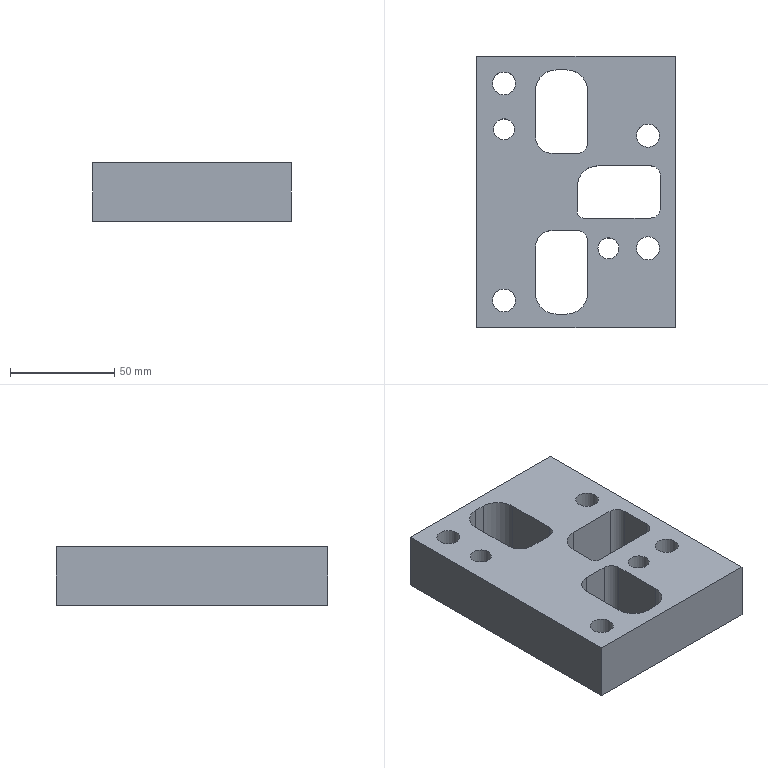Part | STEP file | PN_0015_id866_x_t | 1 solid | 44 faces | box 95 x 130 x 28 mm | volume 241686 mm3 | plane 22 | cylinder 22 | commonest cylinder face diameters 10 x6 20 x5 11 x4 17 x4 16 x2 6 x1
STEP:
#1=CARTESIAN_POINT('',(-190.55,-65.,95.));
#2=VERTEX_POINT('',#1);
#3=CARTESIAN_POINT('',(-190.55,65.,95.));
#4=VERTEX_POINT('',#3);
#5=CARTESIAN_POINT('',(-190.55,0.,95.));
#6=DIRECTION('',(0.,1.,0.));
#7=VECTOR('',#6,1.);
#8=LINE('',#5,#7);
#9=EDGE_CURVE('',#2,#4,#8,.T.);
#10=ORIENTED_EDGE('',*,*,#9,.F.);
#11=CARTESIAN_POINT('',(-190.55,-65.,67.));
#12=VERTEX_POINT('',#11);
#13=CARTESIAN_POINT('',(-190.55,-65.,-36.));
#14=DIRECTION('',(0.,0.,1.));
#15=VECTOR('',#14,1.);
#16=LINE('',#13,#15);
#17=EDGE_CURVE('',#12,#2,#16,.T.);
#18=ORIENTED_EDGE('',*,*,#17,.F.);
#19=CARTESIAN_POINT('',(-190.55,65.,67.));
#20=VERTEX_POINT('',#19);
#21=CARTESIAN_POINT('',(-190.55,0.,67.));
#22=DIRECTION('',(0.,1.,0.));
#23=VECTOR('',#22,1.);
#24=LINE('',#21,#23);
#25=EDGE_CURVE('',#12,#20,#24,.T.);
#26=ORIENTED_EDGE('',*,*,#25,.T.);
#27=CARTESIAN_POINT('',(-190.55,65.,-36.));
#28=DIRECTION('',(0.,0.,1.));
#29=VECTOR('',#28,1.);
#30=LINE('',#27,#29);
#31=EDGE_CURVE('',#20,#4,#30,.T.);
#32=ORIENTED_EDGE('',*,*,#31,.T.);
#33=EDGE_LOOP('',(#10,#18,#26,#32));
#34=FACE_OUTER_BOUND('',#33,.T.);
#35=CARTESIAN_POINT('',(-190.55,0.,-36.));
#36=DIRECTION('',(-1.,0.,0.));
#37=DIRECTION('',(0.,1.,0.));
#38=AXIS2_PLACEMENT_3D('',#35,#36,#37);
#39=PLANE('',#38);
#40=ADVANCED_FACE('',(#34),#39,.F.);
#41=CARTESIAN_POINT('',(-285.55,-65.,67.));
#42=VERTEX_POINT('',#41);
#43=CARTESIAN_POINT('',(-224.,-65.,67.));
#44=DIRECTION('',(1.,0.,0.));
#45=VECTOR('',#44,1.);
#46=LINE('',#43,#45);
#47=EDGE_CURVE('',#42,#12,#46,.T.);
#48=ORIENTED_EDGE('',*,*,#47,.T.);
#49=ORIENTED_EDGE('',*,*,#17,.T.);
#50=CARTESIAN_POINT('',(-285.55,-65.,95.));
#51=VERTEX_POINT('',#50);
#52=CARTESIAN_POINT('',(-224.,-65.,95.));
#53=DIRECTION('',(1.,0.,0.));
#54=VECTOR('',#53,1.);
#55=LINE('',#52,#54);
#56=EDGE_CURVE('',#51,#2,#55,.T.);
#57=ORIENTED_EDGE('',*,*,#56,.F.);
#58=CARTESIAN_POINT('',(-285.55,-65.,-36.));
#59=DIRECTION('',(0.,0.,1.));
#60=VECTOR('',#59,1.);
#61=LINE('',#58,#60);
#62=EDGE_CURVE('',#42,#51,#61,.T.);
#63=ORIENTED_EDGE('',*,*,#62,.F.);
#64=EDGE_LOOP('',(#48,#49,#57,#63));
#65=FACE_OUTER_BOUND('',#64,.T.);
#66=CARTESIAN_POINT('',(-224.,-65.,-36.));
#67=DIRECTION('',(0.,-1.,0.));
#68=DIRECTION('',(-1.,0.,0.));
#69=AXIS2_PLACEMENT_3D('',#66,#67,#68);
#70=PLANE('',#69);
#71=ADVANCED_FACE('',(#65),#70,.T.);
#72=ORIENTED_EDGE('',*,*,#56,.T.);
#73=ORIENTED_EDGE('',*,*,#9,.T.);
#74=CARTESIAN_POINT('',(-285.55,65.,95.));
#75=VERTEX_POINT('',#74);
#76=CARTESIAN_POINT('',(-119.811,65.,95.));
#77=DIRECTION('',(1.,0.,0.));
#78=VECTOR('',#77,1.);
#79=LINE('',#76,#78);
#80=EDGE_CURVE('',#75,#4,#79,.T.);
#81=ORIENTED_EDGE('',*,*,#80,.F.);
#82=CARTESIAN_POINT('',(-285.55,0.,95.));
#83=DIRECTION('',(0.,-1.,0.));
#84=VECTOR('',#83,1.);
#85=LINE('',#82,#84);
#86=EDGE_CURVE('',#75,#51,#85,.T.);
#87=ORIENTED_EDGE('',*,*,#86,.T.);
#88=EDGE_LOOP('',(#72,#73,#81,#87));
#89=FACE_BOUND('',#88,.T.);
#90=CARTESIAN_POINT('',(-267.05,52.,95.));
#91=VERTEX_POINT('',#90);
#92=CARTESIAN_POINT('',(-272.55,52.,95.));
#93=DIRECTION('',(0.,0.,-1.));
#94=DIRECTION('',(1.,0.,0.));
#95=AXIS2_PLACEMENT_3D('',#92,#93,#94);
#96=CIRCLE('',#95,5.5);
#97=EDGE_CURVE('',#91,#91,#96,.T.);
#98=ORIENTED_EDGE('',*,*,#97,.T.);
#99=EDGE_LOOP('',(#98));
#100=FACE_BOUND('',#99,.T.);
#101=CARTESIAN_POINT('',(-267.05,-52.,95.));
#102=VERTEX_POINT('',#101);
#103=CARTESIAN_POINT('',(-272.55,-52.,95.));
#104=DIRECTION('',(0.,0.,-1.));
#105=DIRECTION('',(1.,0.,0.));
#106=AXIS2_PLACEMENT_3D('',#103,#104,#105);
#107=CIRCLE('',#106,5.5);
#108=EDGE_CURVE('',#102,#102,#107,.T.);
#109=ORIENTED_EDGE('',*,*,#108,.T.);
#110=EDGE_LOOP('',(#109));
#111=FACE_BOUND('',#110,.T.);
#112=CARTESIAN_POINT('',(-198.05,-27.,95.));
#113=VERTEX_POINT('',#112);
#114=CARTESIAN_POINT('',(-203.55,-27.,95.));
#115=DIRECTION('',(0.,0.,-1.));
#116=DIRECTION('',(1.,0.,0.));
#117=AXIS2_PLACEMENT_3D('',#114,#115,#116);
#118=CIRCLE('',#117,5.5);
#119=EDGE_CURVE('',#113,#113,#118,.T.);
#120=ORIENTED_EDGE('',*,*,#119,.T.);
#121=EDGE_LOOP('',(#120));
#122=FACE_BOUND('',#121,.T.);
#123=CARTESIAN_POINT('',(-198.05,27.,95.));
#124=VERTEX_POINT('',#123);
#125=CARTESIAN_POINT('',(-203.55,27.,95.));
#126=DIRECTION('',(0.,0.,-1.));
#127=DIRECTION('',(1.,0.,0.));
#128=AXIS2_PLACEMENT_3D('',#125,#126,#127);
#129=CIRCLE('',#128,5.5);
#130=EDGE_CURVE('',#124,#124,#129,.T.);
#131=ORIENTED_EDGE('',*,*,#130,.T.);
#132=EDGE_LOOP('',(#131));
#133=FACE_BOUND('',#132,.T.);
#134=CARTESIAN_POINT('',(-227.5,12.5,95.));
#135=VERTEX_POINT('',#134);
#136=CARTESIAN_POINT('',(-237.5,2.5,95.));
#137=VERTEX_POINT('',#136);
#138=CARTESIAN_POINT('',(-227.5,2.5,95.));
#139=DIRECTION('',(0.,0.,1.));
#140=DIRECTION('',(1.,0.,0.));
#141=AXIS2_PLACEMENT_3D('',#138,#139,#140);
#142=CIRCLE('',#141,10.);
#143=EDGE_CURVE('',#135,#137,#142,.T.);
#144=ORIENTED_EDGE('',*,*,#143,.F.);
#145=CARTESIAN_POINT('',(-202.5,12.5,95.));
#146=VERTEX_POINT('',#145);
#147=CARTESIAN_POINT('',(-209.,12.5,95.));
#148=DIRECTION('',(1.,0.,0.));
#149=VECTOR('',#148,1.);
#150=LINE('',#147,#149);
#151=EDGE_CURVE('',#135,#146,#150,.T.);
#152=ORIENTED_EDGE('',*,*,#151,.T.);
#153=CARTESIAN_POINT('',(-197.5,7.5,95.));
#154=VERTEX_POINT('',#153);
#155=CARTESIAN_POINT('',(-202.5,7.5,95.));
#156=DIRECTION('',(0.,0.,1.));
#157=DIRECTION('',(1.,0.,0.));
#158=AXIS2_PLACEMENT_3D('',#155,#156,#157);
#159=CIRCLE('',#158,5.);
#160=EDGE_CURVE('',#154,#146,#159,.T.);
#161=ORIENTED_EDGE('',*,*,#160,.F.);
#162=CARTESIAN_POINT('',(-197.5,-7.5,95.));
#163=VERTEX_POINT('',#162);
#164=CARTESIAN_POINT('',(-197.5,0.,95.));
#165=DIRECTION('',(0.,-1.,0.));
#166=VECTOR('',#165,1.);
#167=LINE('',#164,#166);
#168=EDGE_CURVE('',#154,#163,#167,.T.);
#169=ORIENTED_EDGE('',*,*,#168,.T.);
#170=CARTESIAN_POINT('',(-202.5,-12.5,95.));
#171=VERTEX_POINT('',#170);
#172=CARTESIAN_POINT('',(-202.5,-7.5,95.));
#173=DIRECTION('',(0.,0.,1.));
#174=DIRECTION('',(1.,0.,0.));
#175=AXIS2_PLACEMENT_3D('',#172,#173,#174);
#176=CIRCLE('',#175,5.);
#177=EDGE_CURVE('',#171,#163,#176,.T.);
#178=ORIENTED_EDGE('',*,*,#177,.F.);
#179=CARTESIAN_POINT('',(-234.5,-12.5,95.));
#180=VERTEX_POINT('',#179);
#181=CARTESIAN_POINT('',(-209.,-12.5,95.));
#182=DIRECTION('',(-1.,0.,0.));
#183=VECTOR('',#182,1.);
#184=LINE('',#181,#183);
#185=EDGE_CURVE('',#171,#180,#184,.T.);
#186=ORIENTED_EDGE('',*,*,#185,.T.);
#187=CARTESIAN_POINT('',(-237.5,-9.5,95.));
#188=VERTEX_POINT('',#187);
#189=CARTESIAN_POINT('',(-234.5,-9.5,95.));
#190=DIRECTION('',(0.,0.,1.));
#191=DIRECTION('',(1.,0.,0.));
#192=AXIS2_PLACEMENT_3D('',#189,#190,#191);
#193=CIRCLE('',#192,3.);
#194=EDGE_CURVE('',#188,#180,#193,.T.);
#195=ORIENTED_EDGE('',*,*,#194,.F.);
#196=CARTESIAN_POINT('',(-237.5,0.,95.));
#197=DIRECTION('',(0.,1.,0.));
#198=VECTOR('',#197,1.);
#199=LINE('',#196,#198);
#200=EDGE_CURVE('',#188,#137,#199,.T.);
#201=ORIENTED_EDGE('',*,*,#200,.T.);
#202=EDGE_LOOP('',(#144,#152,#161,#169,#178,#186,#195,#201));
#203=FACE_BOUND('',#202,.T.);
#204=CARTESIAN_POINT('',(-237.5,18.5,95.));
#205=VERTEX_POINT('',#204);
#206=CARTESIAN_POINT('',(-232.5,23.5,95.));
#207=VERTEX_POINT('',#206);
#208=CARTESIAN_POINT('',(-237.5,23.5,95.));
#209=DIRECTION('',(0.,0.,1.));
#210=DIRECTION('',(1.,0.,0.));
#211=AXIS2_PLACEMENT_3D('',#208,#209,#210);
#212=CIRCLE('',#211,5.);
#213=EDGE_CURVE('',#205,#207,#212,.T.);
#214=ORIENTED_EDGE('',*,*,#213,.F.);
#215=CARTESIAN_POINT('',(-249.5,18.5,95.));
#216=VERTEX_POINT('',#215);
#217=CARTESIAN_POINT('',(-245.,18.5,95.));
#218=DIRECTION('',(-1.,0.,0.));
#219=VECTOR('',#218,1.);
#220=LINE('',#217,#219);
#221=EDGE_CURVE('',#205,#216,#220,.T.);
#222=ORIENTED_EDGE('',*,*,#221,.T.);
#223=CARTESIAN_POINT('',(-257.5,26.5,95.));
#224=VERTEX_POINT('',#223);
#225=CARTESIAN_POINT('',(-249.5,26.5,95.));
#226=DIRECTION('',(0.,0.,1.));
#227=DIRECTION('',(1.,0.,0.));
#228=AXIS2_PLACEMENT_3D('',#225,#226,#227);
#229=CIRCLE('',#228,8.);
#230=EDGE_CURVE('',#224,#216,#229,.T.);
#231=ORIENTED_EDGE('',*,*,#230,.F.);
#232=CARTESIAN_POINT('',(-257.5,48.5,95.));
#233=VERTEX_POINT('',#232);
#234=CARTESIAN_POINT('',(-257.5,47.,95.));
#235=DIRECTION('',(0.,1.,0.));
#236=VECTOR('',#235,1.);
#237=LINE('',#234,#236);
#238=EDGE_CURVE('',#224,#233,#237,.T.);
#239=ORIENTED_EDGE('',*,*,#238,.T.);
#240=CARTESIAN_POINT('',(-247.5,58.5,95.));
#241=VERTEX_POINT('',#240);
#242=CARTESIAN_POINT('',(-247.5,48.5,95.));
#243=DIRECTION('',(0.,0.,1.));
#244=DIRECTION('',(1.,0.,0.));
#245=AXIS2_PLACEMENT_3D('',#242,#243,#244);
#246=CIRCLE('',#245,10.);
#247=EDGE_CURVE('',#241,#233,#246,.T.);
#248=ORIENTED_EDGE('',*,*,#247,.F.);
#249=CARTESIAN_POINT('',(-242.5,58.5,95.));
#250=VERTEX_POINT('',#249);
#251=CARTESIAN_POINT('',(-245.,58.5,95.));
#252=DIRECTION('',(1.,0.,0.));
#253=VECTOR('',#252,1.);
#254=LINE('',#251,#253);
#255=EDGE_CURVE('',#241,#250,#254,.T.);
#256=ORIENTED_EDGE('',*,*,#255,.T.);
#257=CARTESIAN_POINT('',(-232.5,48.5,95.));
#258=VERTEX_POINT('',#257);
#259=CARTESIAN_POINT('',(-242.5,48.5,95.));
#260=DIRECTION('',(0.,0.,1.));
#261=DIRECTION('',(1.,0.,0.));
#262=AXIS2_PLACEMENT_3D('',#259,#260,#261);
#263=CIRCLE('',#262,10.);
#264=EDGE_CURVE('',#258,#250,#263,.T.);
#265=ORIENTED_EDGE('',*,*,#264,.F.);
#266=CARTESIAN_POINT('',(-232.5,47.,95.));
#267=DIRECTION('',(0.,-1.,0.));
#268=VECTOR('',#267,1.);
#269=LINE('',#266,#268);
#270=EDGE_CURVE('',#258,#207,#269,.T.);
#271=ORIENTED_EDGE('',*,*,#270,.T.);
#272=EDGE_LOOP('',(#214,#222,#231,#239,#248,#256,#265,#271));
#273=FACE_BOUND('',#272,.T.);
#274=CARTESIAN_POINT('',(-247.5,-58.5,95.));
#275=VERTEX_POINT('',#274);
#276=CARTESIAN_POINT('',(-242.5,-58.5,95.));
#277=VERTEX_POINT('',#276);
#278=CARTESIAN_POINT('',(-245.,-58.5,95.));
#279=DIRECTION('',(1.,0.,0.));
#280=VECTOR('',#279,1.);
#281=LINE('',#278,#280);
#282=EDGE_CURVE('',#275,#277,#281,.T.);
#283=ORIENTED_EDGE('',*,*,#282,.F.);
#284=CARTESIAN_POINT('',(-257.5,-48.5,95.));
#285=VERTEX_POINT('',#284);
#286=CARTESIAN_POINT('',(-247.5,-48.5,95.));
#287=DIRECTION('',(0.,0.,-1.));
#288=DIRECTION('',(1.,0.,0.));
#289=AXIS2_PLACEMENT_3D('',#286,#287,#288);
#290=CIRCLE('',#289,10.);
#291=EDGE_CURVE('',#275,#285,#290,.T.);
#292=ORIENTED_EDGE('',*,*,#291,.T.);
#293=CARTESIAN_POINT('',(-257.5,-26.5,95.));
#294=VERTEX_POINT('',#293);
#295=CARTESIAN_POINT('',(-257.5,-47.,95.));
#296=DIRECTION('',(0.,-1.,0.));
#297=VECTOR('',#296,1.);
#298=LINE('',#295,#297);
#299=EDGE_CURVE('',#294,#285,#298,.T.);
#300=ORIENTED_EDGE('',*,*,#299,.F.);
#301=CARTESIAN_POINT('',(-249.5,-18.5,95.));
#302=VERTEX_POINT('',#301);
#303=CARTESIAN_POINT('',(-249.5,-26.5,95.));
#304=DIRECTION('',(0.,0.,-1.));
#305=DIRECTION('',(1.,0.,0.));
#306=AXIS2_PLACEMENT_3D('',#303,#304,#305);
#307=CIRCLE('',#306,8.);
#308=EDGE_CURVE('',#294,#302,#307,.T.);
#309=ORIENTED_EDGE('',*,*,#308,.T.);
#310=CARTESIAN_POINT('',(-237.5,-18.5,95.));
#311=VERTEX_POINT('',#310);
#312=CARTESIAN_POINT('',(-245.,-18.5,95.));
#313=DIRECTION('',(-1.,0.,0.));
#314=VECTOR('',#313,1.);
#315=LINE('',#312,#314);
#316=EDGE_CURVE('',#311,#302,#315,.T.);
#317=ORIENTED_EDGE('',*,*,#316,.F.);
#318=CARTESIAN_POINT('',(-232.5,-23.5,95.));
#319=VERTEX_POINT('',#318);
#320=CARTESIAN_POINT('',(-237.5,-23.5,95.));
#321=DIRECTION('',(0.,0.,-1.));
#322=DIRECTION('',(1.,0.,0.));
#323=AXIS2_PLACEMENT_3D('',#320,#321,#322);
#324=CIRCLE('',#323,5.);
#325=EDGE_CURVE('',#311,#319,#324,.T.);
#326=ORIENTED_EDGE('',*,*,#325,.T.);
#327=CARTESIAN_POINT('',(-232.5,-48.5,95.));
#328=VERTEX_POINT('',#327);
#329=CARTESIAN_POINT('',(-232.5,-47.,95.));
#330=DIRECTION('',(0.,1.,0.));
#331=VECTOR('',#330,1.);
#332=LINE('',#329,#331);
#333=EDGE_CURVE('',#328,#319,#332,.T.);
#334=ORIENTED_EDGE('',*,*,#333,.F.);
#335=CARTESIAN_POINT('',(-242.5,-48.5,95.));
#336=DIRECTION('',(0.,0.,-1.));
#337=DIRECTION('',(1.,0.,0.));
#338=AXIS2_PLACEMENT_3D('',#335,#336,#337);
#339=CIRCLE('',#338,10.);
#340=EDGE_CURVE('',#328,#277,#339,.T.);
#341=ORIENTED_EDGE('',*,*,#340,.T.);
#342=EDGE_LOOP('',(#283,#292,#300,#309,#317,#326,#334,#341));
#343=FACE_BOUND('',#342,.T.);
#344=CARTESIAN_POINT('',(-277.55,30.,95.));
#345=VERTEX_POINT('',#344);
#346=CARTESIAN_POINT('',(-272.55,30.,95.));
#347=DIRECTION('',(0.,0.,1.));
#348=DIRECTION('',(-1.,0.,0.));
#349=AXIS2_PLACEMENT_3D('',#346,#347,#348);
#350=CIRCLE('',#349,5.);
#351=EDGE_CURVE('',#345,#345,#350,.T.);
#352=ORIENTED_EDGE('',*,*,#351,.F.);
#353=EDGE_LOOP('',(#352));
#354=FACE_BOUND('',#353,.T.);
#355=CARTESIAN_POINT('',(-227.55,-27.,95.));
#356=VERTEX_POINT('',#355);
#357=CARTESIAN_POINT('',(-222.55,-27.,95.));
#358=DIRECTION('',(0.,0.,1.));
#359=DIRECTION('',(-1.,0.,0.));
#360=AXIS2_PLACEMENT_3D('',#357,#358,#359);
#361=CIRCLE('',#360,5.);
#362=EDGE_CURVE('',#356,#356,#361,.T.);
#363=ORIENTED_EDGE('',*,*,#362,.F.);
#364=EDGE_LOOP('',(#363));
#365=FACE_BOUND('',#364,.T.);
#366=CARTESIAN_POINT('',(-119.811,64.,95.));
#367=DIRECTION('',(0.,0.,1.));
#368=DIRECTION('',(1.,0.,0.));
#369=AXIS2_PLACEMENT_3D('',#366,#367,#368);
#370=PLANE('',#369);
#371=ADVANCED_FACE('',(#89,#100,#111,#122,#133,#203,#273,#343,#354,#365),#370,.T.);
#372=ORIENTED_EDGE('',*,*,#25,.F.);
#373=ORIENTED_EDGE('',*,*,#47,.F.);
#374=CARTESIAN_POINT('',(-285.55,65.,67.));
#375=VERTEX_POINT('',#374);
#376=CARTESIAN_POINT('',(-285.55,0.,67.));
#377=DIRECTION('',(0.,-1.,0.));
#378=VECTOR('',#377,1.);
#379=LINE('',#376,#378);
#380=EDGE_CURVE('',#375,#42,#379,.T.);
#381=ORIENTED_EDGE('',*,*,#380,.F.);
#382=CARTESIAN_POINT('',(-119.811,65.,67.));
#383=DIRECTION('',(1.,0.,0.));
#384=VECTOR('',#383,1.);
#385=LINE('',#382,#384);
#386=EDGE_CURVE('',#375,#20,#385,.T.);
#387=ORIENTED_EDGE('',*,*,#386,.T.);
#388=EDGE_LOOP('',(#372,#373,#381,#387));
#389=FACE_BOUND('',#388,.T.);
#390=CARTESIAN_POINT('',(-227.55,-27.,67.));
#391=VERTEX_POINT('',#390);
#392=CARTESIAN_POINT('',(-222.55,-27.,67.));
#393=DIRECTION('',(0.,0.,1.));
#394=DIRECTION('',(-1.,0.,0.));
#395=AXIS2_PLACEMENT_3D('',#392,#393,#394);
#396=CIRCLE('',#395,5.);
#397=EDGE_CURVE('',#391,#391,#396,.T.);
#398=ORIENTED_EDGE('',*,*,#397,.T.);
#399=EDGE_LOOP('',(#398));
#400=FACE_BOUND('',#399,.T.);
#401=CARTESIAN_POINT('',(-277.55,30.,67.));
#402=VERTEX_POINT('',#401);
#403=CARTESIAN_POINT('',(-272.55,30.,67.));
#404=DIRECTION('',(0.,0.,1.));
#405=DIRECTION('',(-1.,0.,0.));
#406=AXIS2_PLACEMENT_3D('',#403,#404,#405);
#407=CIRCLE('',#406,5.);
#408=EDGE_CURVE('',#402,#402,#407,.T.);
#409=ORIENTED_EDGE('',*,*,#408,.T.);
#410=EDGE_LOOP('',(#409));
#411=FACE_BOUND('',#410,.T.);
#412=CARTESIAN_POINT('',(-264.05,52.,67.));
#413=VERTEX_POINT('',#412);
#414=CARTESIAN_POINT('',(-272.55,52.,67.));
#415=DIRECTION('',(0.,0.,1.));
#416=DIRECTION('',(1.,0.,0.));
#417=AXIS2_PLACEMENT_3D('',#414,#415,#416);
#418=CIRCLE('',#417,8.5);
#419=EDGE_CURVE('',#413,#413,#418,.T.);
#420=ORIENTED_EDGE('',*,*,#419,.T.);
#421=EDGE_LOOP('',(#420));
#422=FACE_BOUND('',#421,.T.);
#423=CARTESIAN_POINT('',(-264.05,-52.,67.));
#424=VERTEX_POINT('',#423);
#425=CARTESIAN_POINT('',(-272.55,-52.,67.));
#426=DIRECTION('',(0.,0.,-1.));
#427=DIRECTION('',(1.,0.,0.));
#428=AXIS2_PLACEMENT_3D('',#425,#426,#427);
#429=CIRCLE('',#428,8.5);
#430=EDGE_CURVE('',#424,#424,#429,.T.);
#431=ORIENTED_EDGE('',*,*,#430,.F.);
#432=EDGE_LOOP('',(#431));
#433=FACE_BOUND('',#432,.T.);
#434=CARTESIAN_POINT('',(-195.05,-27.,67.));
#435=VERTEX_POINT('',#434);
#436=CARTESIAN_POINT('',(-203.55,-27.,67.));
#437=DIRECTION('',(0.,0.,-1.));
#438=DIRECTION('',(1.,0.,0.));
#439=AXIS2_PLACEMENT_3D('',#436,#437,#438);
#440=CIRCLE('',#439,8.5);
#441=EDGE_CURVE('',#435,#435,#440,.T.);
#442=ORIENTED_EDGE('',*,*,#441,.F.);
#443=EDGE_LOOP('',(#442));
#444=FACE_BOUND('',#443,.T.);
#445=CARTESIAN_POINT('',(-195.05,27.,67.));
#446=VERTEX_POINT('',#445);
#447=CARTESIAN_POINT('',(-203.55,27.,67.));
#448=DIRECTION('',(0.,0.,1.));
#449=DIRECTION('',(1.,0.,0.));
#450=AXIS2_PLACEMENT_3D('',#447,#448,#449);
#451=CIRCLE('',#450,8.5);
#452=EDGE_CURVE('',#446,#446,#451,.T.);
#453=ORIENTED_EDGE('',*,*,#452,.T.);
#454=EDGE_LOOP('',(#453));
#455=FACE_BOUND('',#454,.T.);
#456=CARTESIAN_POINT('',(-227.5,12.5,67.));
#457=VERTEX_POINT('',#456);
#458=CARTESIAN_POINT('',(-202.5,12.5,67.));
#459=VERTEX_POINT('',#458);
#460=CARTESIAN_POINT('',(-119.811,12.5,67.));
#461=DIRECTION('',(1.,0.,0.));
#462=VECTOR('',#461,1.);
#463=LINE('',#460,#462);
#464=EDGE_CURVE('',#457,#459,#463,.T.);
#465=ORIENTED_EDGE('',*,*,#464,.F.);
#466=CARTESIAN_POINT('',(-237.5,2.5,67.));
#467=VERTEX_POINT('',#466);
#468=CARTESIAN_POINT('',(-227.5,2.5,67.));
#469=DIRECTION('',(0.,0.,-1.));
#470=DIRECTION('',(1.,0.,0.));
#471=AXIS2_PLACEMENT_3D('',#468,#469,#470);
#472=CIRCLE('',#471,10.);
#473=EDGE_CURVE('',#467,#457,#472,.T.);
#474=ORIENTED_EDGE('',*,*,#473,.F.);
#475=CARTESIAN_POINT('',(-237.5,-9.5,67.));
#476=VERTEX_POINT('',#475);
#477=CARTESIAN_POINT('',(-237.5,64.,67.));
#478=DIRECTION('',(0.,1.,0.));
#479=VECTOR('',#478,1.);
#480=LINE('',#477,#479);
#481=EDGE_CURVE('',#476,#467,#480,.T.);
#482=ORIENTED_EDGE('',*,*,#481,.F.);
#483=CARTESIAN_POINT('',(-234.5,-12.5,67.));
#484=VERTEX_POINT('',#483);
#485=CARTESIAN_POINT('',(-234.5,-9.5,67.));
#486=DIRECTION('',(0.,0.,-1.));
#487=DIRECTION('',(1.,0.,0.));
#488=AXIS2_PLACEMENT_3D('',#485,#486,#487);
#489=CIRCLE('',#488,3.);
#490=EDGE_CURVE('',#484,#476,#489,.T.);
#491=ORIENTED_EDGE('',*,*,#490,.F.);
#492=CARTESIAN_POINT('',(-202.5,-12.5,67.));
#493=VERTEX_POINT('',#492);
#494=CARTESIAN_POINT('',(-119.811,-12.5,67.));
#495=DIRECTION('',(-1.,0.,0.));
#496=VECTOR('',#495,1.);
#497=LINE('',#494,#496);
#498=EDGE_CURVE('',#493,#484,#497,.T.);
#499=ORIENTED_EDGE('',*,*,#498,.F.);
#500=CARTESIAN_POINT('',(-197.5,-7.5,67.));
#501=VERTEX_POINT('',#500);
#502=CARTESIAN_POINT('',(-202.5,-7.5,67.));
#503=DIRECTION('',(0.,0.,-1.));
#504=DIRECTION('',(1.,0.,0.));
#505=AXIS2_PLACEMENT_3D('',#502,#503,#504);
#506=CIRCLE('',#505,5.);
#507=EDGE_CURVE('',#501,#493,#506,.T.);
#508=ORIENTED_EDGE('',*,*,#507,.F.);
#509=CARTESIAN_POINT('',(-197.5,7.5,67.));
#510=VERTEX_POINT('',#509);
#511=CARTESIAN_POINT('',(-197.5,64.,67.));
#512=DIRECTION('',(0.,-1.,0.));
#513=VECTOR('',#512,1.);
#514=LINE('',#511,#513);
#515=EDGE_CURVE('',#510,#501,#514,.T.);
#516=ORIENTED_EDGE('',*,*,#515,.F.);
#517=CARTESIAN_POINT('',(-202.5,7.5,67.));
#518=DIRECTION('',(0.,0.,-1.));
#519=DIRECTION('',(1.,0.,0.));
#520=AXIS2_PLACEMENT_3D('',#517,#518,#519);
#521=CIRCLE('',#520,5.);
#522=EDGE_CURVE('',#459,#510,#521,.T.);
#523=ORIENTED_EDGE('',*,*,#522,.F.);
#524=EDGE_LOOP('',(#465,#474,#482,#491,#499,#508,#516,#523));
#525=FACE_BOUND('',#524,.T.);
#526=CARTESIAN_POINT('',(-232.5,-48.5,67.));
#527=VERTEX_POINT('',#526);
#528=CARTESIAN_POINT('',(-242.5,-58.5,67.));
#529=VERTEX_POINT('',#528);
#530=CARTESIAN_POINT('',(-242.5,-48.5,67.));
#531=DIRECTION('',(0.,0.,-1.));
#532=DIRECTION('',(1.,0.,0.));
#533=AXIS2_PLACEMENT_3D('',#530,#531,#532);
#534=CIRCLE('',#533,10.);
#535=EDGE_CURVE('',#527,#529,#534,.T.);
#536=ORIENTED_EDGE('',*,*,#535,.F.);
#537=CARTESIAN_POINT('',(-232.5,-23.5,67.));
#538=VERTEX_POINT('',#537);
#539=CARTESIAN_POINT('',(-232.5,64.,67.));
#540=DIRECTION('',(0.,-1.,0.));
#541=VECTOR('',#540,1.);
#542=LINE('',#539,#541);
#543=EDGE_CURVE('',#538,#527,#542,.T.);
#544=ORIENTED_EDGE('',*,*,#543,.F.);
#545=CARTESIAN_POINT('',(-237.5,-18.5,67.));
#546=VERTEX_POINT('',#545);
#547=CARTESIAN_POINT('',(-237.5,-23.5,67.));
#548=DIRECTION('',(0.,0.,-1.));
#549=DIRECTION('',(1.,0.,0.));
#550=AXIS2_PLACEMENT_3D('',#547,#548,#549);
#551=CIRCLE('',#550,5.);
#552=EDGE_CURVE('',#546,#538,#551,.T.);
#553=ORIENTED_EDGE('',*,*,#552,.F.);
#554=CARTESIAN_POINT('',(-249.5,-18.5,67.));
#555=VERTEX_POINT('',#554);
#556=CARTESIAN_POINT('',(-119.811,-18.5,67.));
#557=DIRECTION('',(1.,0.,0.));
#558=VECTOR('',#557,1.);
#559=LINE('',#556,#558);
#560=EDGE_CURVE('',#555,#546,#559,.T.);
#561=ORIENTED_EDGE('',*,*,#560,.F.);
#562=CARTESIAN_POINT('',(-257.5,-26.5,67.));
#563=VERTEX_POINT('',#562);
#564=CARTESIAN_POINT('',(-249.5,-26.5,67.));
#565=DIRECTION('',(0.,0.,-1.));
#566=DIRECTION('',(1.,0.,0.));
#567=AXIS2_PLACEMENT_3D('',#564,#565,#566);
#568=CIRCLE('',#567,8.);
#569=EDGE_CURVE('',#563,#555,#568,.T.);
#570=ORIENTED_EDGE('',*,*,#569,.F.);
#571=CARTESIAN_POINT('',(-257.5,-48.5,67.));
#572=VERTEX_POINT('',#571);
#573=CARTESIAN_POINT('',(-257.5,64.,67.));
#574=DIRECTION('',(0.,1.,0.));
#575=VECTOR('',#574,1.);
#576=LINE('',#573,#575);
#577=EDGE_CURVE('',#572,#563,#576,.T.);
#578=ORIENTED_EDGE('',*,*,#577,.F.);
#579=CARTESIAN_POINT('',(-247.5,-58.5,67.));
#580=VERTEX_POINT('',#579);
#581=CARTESIAN_POINT('',(-247.5,-48.5,67.));
#582=DIRECTION('',(0.,0.,-1.));
#583=DIRECTION('',(1.,0.,0.));
#584=AXIS2_PLACEMENT_3D('',#581,#582,#583);
#585=CIRCLE('',#584,10.);
#586=EDGE_CURVE('',#580,#572,#585,.T.);
#587=ORIENTED_EDGE('',*,*,#586,.F.);
#588=CARTESIAN_POINT('',(-119.811,-58.5,67.));
#589=DIRECTION('',(-1.,0.,0.));
#590=VECTOR('',#589,1.);
#591=LINE('',#588,#590);
#592=EDGE_CURVE('',#529,#580,#591,.T.);
#593=ORIENTED_EDGE('',*,*,#592,.F.);
#594=EDGE_LOOP('',(#536,#544,#553,#561,#570,#578,#587,#593));
#595=FACE_BOUND('',#594,.T.);
#596=CARTESIAN_POINT('',(-242.5,58.5,67.));
#597=VERTEX_POINT('',#596);
#598=CARTESIAN_POINT('',(-232.5,48.5,67.));
#599=VERTEX_POINT('',#598);
#600=CARTESIAN_POINT('',(-242.5,48.5,67.));
#601=DIRECTION('',(0.,0.,-1.));
#602=DIRECTION('',(1.,0.,0.));
#603=AXIS2_PLACEMENT_3D('',#600,#601,#602);
#604=CIRCLE('',#603,10.);
#605=EDGE_CURVE('',#597,#599,#604,.T.);
#606=ORIENTED_EDGE('',*,*,#605,.F.);
#607=CARTESIAN_POINT('',(-247.5,58.5,67.));
#608=VERTEX_POINT('',#607);
#609=CARTESIAN_POINT('',(-119.811,58.5,67.));
#610=DIRECTION('',(1.,0.,0.));
#611=VECTOR('',#610,1.);
#612=LINE('',#609,#611);
#613=EDGE_CURVE('',#608,#597,#612,.T.);
#614=ORIENTED_EDGE('',*,*,#613,.F.);
#615=CARTESIAN_POINT('',(-257.5,48.5,67.));
#616=VERTEX_POINT('',#615);
#617=CARTESIAN_POINT('',(-247.5,48.5,67.));
#618=DIRECTION('',(0.,0.,-1.));
#619=DIRECTION('',(1.,0.,0.));
#620=AXIS2_PLACEMENT_3D('',#617,#618,#619);
#621=CIRCLE('',#620,10.);
#622=EDGE_CURVE('',#616,#608,#621,.T.);
#623=ORIENTED_EDGE('',*,*,#622,.F.);
#624=CARTESIAN_POINT('',(-257.5,26.5,67.));
#625=VERTEX_POINT('',#624);
#626=CARTESIAN_POINT('',(-257.5,64.,67.));
#627=DIRECTION('',(0.,1.,0.));
#628=VECTOR('',#627,1.);
#629=LINE('',#626,#628);
#630=EDGE_CURVE('',#625,#616,#629,.T.);
#631=ORIENTED_EDGE('',*,*,#630,.F.);
#632=CARTESIAN_POINT('',(-249.5,18.5,67.));
#633=VERTEX_POINT('',#632);
#634=CARTESIAN_POINT('',(-249.5,26.5,67.));
#635=DIRECTION('',(0.,0.,-1.));
#636=DIRECTION('',(1.,0.,0.));
#637=AXIS2_PLACEMENT_3D('',#634,#635,#636);
#638=CIRCLE('',#637,8.);
#639=EDGE_CURVE('',#633,#625,#638,.T.);
#640=ORIENTED_EDGE('',*,*,#639,.F.);
#641=CARTESIAN_POINT('',(-237.5,18.5,67.));
#642=VERTEX_POINT('',#641);
#643=CARTESIAN_POINT('',(-119.811,18.5,67.));
#644=DIRECTION('',(-1.,0.,0.));
#645=VECTOR('',#644,1.);
#646=LINE('',#643,#645);
#647=EDGE_CURVE('',#642,#633,#646,.T.);
#648=ORIENTED_EDGE('',*,*,#647,.F.);
#649=CARTESIAN_POINT('',(-232.5,23.5,67.));
#650=VERTEX_POINT('',#649);
#651=CARTESIAN_POINT('',(-237.5,23.5,67.));
#652=DIRECTION('',(0.,0.,-1.));
#653=DIRECTION('',(1.,0.,0.));
#654=AXIS2_PLACEMENT_3D('',#651,#652,#653);
#655=CIRCLE('',#654,5.);
#656=EDGE_CURVE('',#650,#642,#655,.T.);
#657=ORIENTED_EDGE('',*,*,#656,.F.);
#658=CARTESIAN_POINT('',(-232.5,64.,67.));
#659=DIRECTION('',(0.,-1.,0.));
#660=VECTOR('',#659,1.);
#661=LINE('',#658,#660);
#662=EDGE_CURVE('',#599,#650,#661,.T.);
#663=ORIENTED_EDGE('',*,*,#662,.F.);
#664=EDGE_LOOP('',(#606,#614,#623,#631,#640,#648,#657,#663));
#665=FACE_BOUND('',#664,.T.);
#666=CARTESIAN_POINT('',(-119.811,64.,67.));
#667=DIRECTION('',(0.,0.,1.));
#668=DIRECTION('',(1.,0.,0.));
#669=AXIS2_PLACEMENT_3D('',#666,#667,#668);
#670=PLANE('',#669);
#671=ADVANCED_FACE('',(#389,#400,#411,#422,#433,#444,#455,#525,#595,#665),#670,.F.);
#672=ORIENTED_EDGE('',*,*,#151,.F.);
#673=CARTESIAN_POINT('',(-227.5,12.5,5.));
#674=DIRECTION('',(0.,0.,-1.));
#675=VECTOR('',#674,1.);
#676=LINE('',#673,#675);
#677=EDGE_CURVE('',#135,#457,#676,.T.);
#678=ORIENTED_EDGE('',*,*,#677,.T.);
#679=ORIENTED_EDGE('',*,*,#464,.T.);
#680=CARTESIAN_POINT('',(-202.5,12.5,5.));
#681=DIRECTION('',(0.,0.,1.));
#682=VECTOR('',#681,1.);
#683=LINE('',#680,#682);
#684=EDGE_CURVE('',#459,#146,#683,.T.);
#685=ORIENTED_EDGE('',*,*,#684,.T.);
#686=EDGE_LOOP('',(#672,#678,#679,#685));
#687=FACE_OUTER_BOUND('',#686,.T.);
#688=CARTESIAN_POINT('',(-209.,12.5,5.));
#689=DIRECTION('',(0.,1.,0.));
#690=DIRECTION('',(0.,0.,1.));
#691=AXIS2_PLACEMENT_3D('',#688,#689,#690);
#692=PLANE('',#691);
#693=ADVANCED_FACE('',(#687),#692,.F.);
#694=ORIENTED_EDGE('',*,*,#515,.T.);
#695=CARTESIAN_POINT('',(-197.5,-7.5,5.));
#696=DIRECTION('',(0.,0.,1.));
#697=VECTOR('',#696,1.);
#698=LINE('',#695,#697);
#699=EDGE_CURVE('',#501,#163,#698,.T.);
#700=ORIENTED_EDGE('',*,*,#699,.T.);
#701=ORIENTED_EDGE('',*,*,#168,.F.);
#702=CARTESIAN_POINT('',(-197.5,7.5,5.));
#703=DIRECTION('',(0.,0.,-1.));
#704=VECTOR('',#703,1.);
#705=LINE('',#702,#704);
#706=EDGE_CURVE('',#154,#510,#705,.T.);
#707=ORIENTED_EDGE('',*,*,#706,.T.);
#708=EDGE_LOOP('',(#694,#700,#701,#707));
#709=FACE_OUTER_BOUND('',#708,.T.);
#710=CARTESIAN_POINT('',(-197.5,0.,5.));
#711=DIRECTION('',(1.,0.,0.));
#712=DIRECTION('',(0.,0.,1.));
#713=AXIS2_PLACEMENT_3D('',#710,#711,#712);
#714=PLANE('',#713);
#715=ADVANCED_FACE('',(#709),#714,.F.);
#716=ORIENTED_EDGE('',*,*,#498,.T.);
#717=CARTESIAN_POINT('',(-234.5,-12.5,5.));
#718=DIRECTION('',(0.,0.,1.));
#719=VECTOR('',#718,1.);
#720=LINE('',#717,#719);
#721=EDGE_CURVE('',#484,#180,#720,.T.);
#722=ORIENTED_EDGE('',*,*,#721,.T.);
#723=ORIENTED_EDGE('',*,*,#185,.F.);
#724=CARTESIAN_POINT('',(-202.5,-12.5,5.));
#725=DIRECTION('',(0.,0.,-1.));
#726=VECTOR('',#725,1.);
#727=LINE('',#724,#726);
#728=EDGE_CURVE('',#171,#493,#727,.T.);
#729=ORIENTED_EDGE('',*,*,#728,.T.);
#730=EDGE_LOOP('',(#716,#722,#723,#729));
#731=FACE_OUTER_BOUND('',#730,.T.);
#732=CARTESIAN_POINT('',(-209.,-12.5,5.));
#733=DIRECTION('',(0.,-1.,0.));
#734=DIRECTION('',(0.,0.,-1.));
#735=AXIS2_PLACEMENT_3D('',#732,#733,#734);
#736=PLANE('',#735);
#737=ADVANCED_FACE('',(#731),#736,.F.);
#738=ORIENTED_EDGE('',*,*,#507,.T.);
#739=ORIENTED_EDGE('',*,*,#728,.F.);
#740=ORIENTED_EDGE('',*,*,#177,.T.);
#741=ORIENTED_EDGE('',*,*,#699,.F.);
#742=EDGE_LOOP('',(#738,#739,#740,#741));
#743=FACE_OUTER_BOUND('',#742,.T.);
#744=CARTESIAN_POINT('',(-202.5,-7.5,5.));
#745=DIRECTION('',(0.,0.,1.));
#746=DIRECTION('',(1.,0.,0.));
#747=AXIS2_PLACEMENT_3D('',#744,#745,#746);
#748=CYLINDRICAL_SURFACE('',#747,5.);
#749=ADVANCED_FACE('',(#743),#748,.F.);
#750=ORIENTED_EDGE('',*,*,#522,.T.);
#751=ORIENTED_EDGE('',*,*,#706,.F.);
#752=ORIENTED_EDGE('',*,*,#160,.T.);
#753=ORIENTED_EDGE('',*,*,#684,.F.);
#754=EDGE_LOOP('',(#750,#751,#752,#753));
#755=FACE_OUTER_BOUND('',#754,.T.);
#756=CARTESIAN_POINT('',(-202.5,7.5,5.));
#757=DIRECTION('',(0.,0.,1.));
#758=DIRECTION('',(1.,0.,0.));
#759=AXIS2_PLACEMENT_3D('',#756,#757,#758);
#760=CYLINDRICAL_SURFACE('',#759,5.);
#761=ADVANCED_FACE('',(#755),#760,.F.);
#762=ORIENTED_EDGE('',*,*,#380,.T.);
#763=ORIENTED_EDGE('',*,*,#62,.T.);
#764=ORIENTED_EDGE('',*,*,#86,.F.);
#765=CARTESIAN_POINT('',(-285.55,65.,-36.));
#766=DIRECTION('',(0.,0.,1.));
#767=VECTOR('',#766,1.);
#768=LINE('',#765,#767);
#769=EDGE_CURVE('',#375,#75,#768,.T.);
#770=ORIENTED_EDGE('',*,*,#769,.F.);
#771=EDGE_LOOP('',(#762,#763,#764,#770));
#772=FACE_OUTER_BOUND('',#771,.T.);
#773=CARTESIAN_POINT('',(-285.55,0.,-36.));
#774=DIRECTION('',(-1.,0.,0.));
#775=DIRECTION('',(0.,1.,0.));
#776=AXIS2_PLACEMENT_3D('',#773,#774,#775);
#777=PLANE('',#776);
#778=ADVANCED_FACE('',(#772),#777,.T.);
#779=ORIENTED_EDGE('',*,*,#481,.T.);
#780=CARTESIAN_POINT('',(-237.5,2.5,5.));
#781=DIRECTION('',(0.,0.,1.));
#782=VECTOR('',#781,1.);
#783=LINE('',#780,#782);
#784=EDGE_CURVE('',#467,#137,#783,.T.);
#785=ORIENTED_EDGE('',*,*,#784,.T.);
#786=ORIENTED_EDGE('',*,*,#200,.F.);
#787=CARTESIAN_POINT('',(-237.5,-9.5,5.));
#788=DIRECTION('',(0.,0.,-1.));
#789=VECTOR('',#788,1.);
#790=LINE('',#787,#789);
#791=EDGE_CURVE('',#188,#476,#790,.T.);
#792=ORIENTED_EDGE('',*,*,#791,.T.);
#793=EDGE_LOOP('',(#779,#785,#786,#792));
#794=FACE_OUTER_BOUND('',#793,.T.);
#795=CARTESIAN_POINT('',(-237.5,0.,5.));
#796=DIRECTION('',(-1.,0.,0.));
#797=DIRECTION('',(0.,0.,-1.));
#798=AXIS2_PLACEMENT_3D('',#795,#796,#797);
#799=PLANE('',#798);
#800=ADVANCED_FACE('',(#794),#799,.F.);
#801=ORIENTED_EDGE('',*,*,#662,.T.);
#802=CARTESIAN_POINT('',(-232.5,23.5,5.));
#803=DIRECTION('',(0.,0.,1.));
#804=VECTOR('',#803,1.);
#805=LINE('',#802,#804);
#806=EDGE_CURVE('',#650,#207,#805,.T.);
#807=ORIENTED_EDGE('',*,*,#806,.T.);
#808=ORIENTED_EDGE('',*,*,#270,.F.);
#809=CARTESIAN_POINT('',(-232.5,48.5,5.));
#810=DIRECTION('',(0.,0.,-1.));
#811=VECTOR('',#810,1.);
#812=LINE('',#809,#811);
#813=EDGE_CURVE('',#258,#599,#812,.T.);
#814=ORIENTED_EDGE('',*,*,#813,.T.);
#815=EDGE_LOOP('',(#801,#807,#808,#814));
#816=FACE_OUTER_BOUND('',#815,.T.);
#817=CARTESIAN_POINT('',(-232.5,47.,5.));
#818=DIRECTION('',(1.,0.,0.));
#819=DIRECTION('',(0.,0.,-1.));
#820=AXIS2_PLACEMENT_3D('',#817,#818,#819);
#821=PLANE('',#820);
#822=ADVANCED_FACE('',(#816),#821,.F.);
#823=ORIENTED_EDGE('',*,*,#656,.T.);
#824=CARTESIAN_POINT('',(-237.5,18.5,5.));
#825=DIRECTION('',(0.,0.,-1.));
#826=VECTOR('',#825,1.);
#827=LINE('',#824,#826);
#828=EDGE_CURVE('',#205,#642,#827,.T.);
#829=ORIENTED_EDGE('',*,*,#828,.F.);
#830=ORIENTED_EDGE('',*,*,#213,.T.);
#831=ORIENTED_EDGE('',*,*,#806,.F.);
#832=EDGE_LOOP('',(#823,#829,#830,#831));
#833=FACE_OUTER_BOUND('',#832,.T.);
#834=CARTESIAN_POINT('',(-237.5,23.5,5.));
#835=DIRECTION('',(0.,0.,1.));
#836=DIRECTION('',(1.,0.,0.));
#837=AXIS2_PLACEMENT_3D('',#834,#835,#836);
#838=CYLINDRICAL_SURFACE('',#837,5.);
#839=ADVANCED_FACE('',(#833),#838,.F.);
#840=ORIENTED_EDGE('',*,*,#647,.T.);
#841=CARTESIAN_POINT('',(-249.5,18.5,5.));
#842=DIRECTION('',(0.,0.,1.));
#843=VECTOR('',#842,1.);
#844=LINE('',#841,#843);
#845=EDGE_CURVE('',#633,#216,#844,.T.);
#846=ORIENTED_EDGE('',*,*,#845,.T.);
#847=ORIENTED_EDGE('',*,*,#221,.F.);
#848=ORIENTED_EDGE('',*,*,#828,.T.);
#849=EDGE_LOOP('',(#840,#846,#847,#848));
#850=FACE_OUTER_BOUND('',#849,.T.);
#851=CARTESIAN_POINT('',(-245.,18.5,5.));
#852=DIRECTION('',(0.,-1.,0.));
#853=DIRECTION('',(0.,0.,-1.));
#854=AXIS2_PLACEMENT_3D('',#851,#852,#853);
#855=PLANE('',#854);
#856=ADVANCED_FACE('',(#850),#855,.F.);
#857=ORIENTED_EDGE('',*,*,#639,.T.);
#858=CARTESIAN_POINT('',(-257.5,26.5,5.));
#859=DIRECTION('',(0.,0.,-1.));
#860=VECTOR('',#859,1.);
#861=LINE('',#858,#860);
#862=EDGE_CURVE('',#224,#625,#861,.T.);
#863=ORIENTED_EDGE('',*,*,#862,.F.);
#864=ORIENTED_EDGE('',*,*,#230,.T.);
#865=ORIENTED_EDGE('',*,*,#845,.F.);
#866=EDGE_LOOP('',(#857,#863,#864,#865));
#867=FACE_OUTER_BOUND('',#866,.T.);
#868=CARTESIAN_POINT('',(-249.5,26.5,5.));
#869=DIRECTION('',(0.,0.,1.));
#870=DIRECTION('',(1.,0.,0.));
#871=AXIS2_PLACEMENT_3D('',#868,#869,#870);
#872=CYLINDRICAL_SURFACE('',#871,8.);
#873=ADVANCED_FACE('',(#867),#872,.F.);
#874=ORIENTED_EDGE('',*,*,#630,.T.);
#875=CARTESIAN_POINT('',(-257.5,48.5,5.));
#876=DIRECTION('',(0.,0.,1.));
#877=VECTOR('',#876,1.);
#878=LINE('',#875,#877);
#879=EDGE_CURVE('',#616,#233,#878,.T.);
#880=ORIENTED_EDGE('',*,*,#879,.T.);
#881=ORIENTED_EDGE('',*,*,#238,.F.);
#882=ORIENTED_EDGE('',*,*,#862,.T.);
#883=EDGE_LOOP('',(#874,#880,#881,#882));
#884=FACE_OUTER_BOUND('',#883,.T.);
#885=CARTESIAN_POINT('',(-257.5,47.,5.));
#886=DIRECTION('',(-1.,0.,0.));
#887=DIRECTION('',(0.,0.,1.));
#888=AXIS2_PLACEMENT_3D('',#885,#886,#887);
#889=PLANE('',#888);
#890=ADVANCED_FACE('',(#884),#889,.F.);
#891=ORIENTED_EDGE('',*,*,#622,.T.);
#892=CARTESIAN_POINT('',(-247.5,58.5,5.));
#893=DIRECTION('',(0.,0.,-1.));
#894=VECTOR('',#893,1.);
#895=LINE('',#892,#894);
#896=EDGE_CURVE('',#241,#608,#895,.T.);
#897=ORIENTED_EDGE('',*,*,#896,.F.);
#898=ORIENTED_EDGE('',*,*,#247,.T.);
#899=ORIENTED_EDGE('',*,*,#879,.F.);
#900=EDGE_LOOP('',(#891,#897,#898,#899));
#901=FACE_OUTER_BOUND('',#900,.T.);
#902=CARTESIAN_POINT('',(-247.5,48.5,5.));
#903=DIRECTION('',(0.,0.,1.));
#904=DIRECTION('',(1.,0.,0.));
#905=AXIS2_PLACEMENT_3D('',#902,#903,#904);
#906=CYLINDRICAL_SURFACE('',#905,10.);
#907=ADVANCED_FACE('',(#901),#906,.F.);
#908=ORIENTED_EDGE('',*,*,#613,.T.);
#909=CARTESIAN_POINT('',(-242.5,58.5,5.));
#910=DIRECTION('',(0.,0.,1.));
#911=VECTOR('',#910,1.);
#912=LINE('',#909,#911);
#913=EDGE_CURVE('',#597,#250,#912,.T.);
#914=ORIENTED_EDGE('',*,*,#913,.T.);
#915=ORIENTED_EDGE('',*,*,#255,.F.);
#916=ORIENTED_EDGE('',*,*,#896,.T.);
#917=EDGE_LOOP('',(#908,#914,#915,#916));
#918=FACE_OUTER_BOUND('',#917,.T.);
#919=CARTESIAN_POINT('',(-245.,58.5,5.));
#920=DIRECTION('',(0.,1.,0.));
#921=DIRECTION('',(0.,0.,1.));
#922=AXIS2_PLACEMENT_3D('',#919,#920,#921);
#923=PLANE('',#922);
#924=ADVANCED_FACE('',(#918),#923,.F.);
#925=ORIENTED_EDGE('',*,*,#605,.T.);
#926=ORIENTED_EDGE('',*,*,#813,.F.);
#927=ORIENTED_EDGE('',*,*,#264,.T.);
#928=ORIENTED_EDGE('',*,*,#913,.F.);
#929=EDGE_LOOP('',(#925,#926,#927,#928));
#930=FACE_OUTER_BOUND('',#929,.T.);
#931=CARTESIAN_POINT('',(-242.5,48.5,5.));
#932=DIRECTION('',(0.,0.,1.));
#933=DIRECTION('',(1.,0.,0.));
#934=AXIS2_PLACEMENT_3D('',#931,#932,#933);
#935=CYLINDRICAL_SURFACE('',#934,10.);
#936=ADVANCED_FACE('',(#930),#935,.F.);
#937=ORIENTED_EDGE('',*,*,#592,.T.);
#938=CARTESIAN_POINT('',(-247.5,-58.5,5.));
#939=DIRECTION('',(0.,0.,-1.));
#940=VECTOR('',#939,1.);
#941=LINE('',#938,#940);
#942=EDGE_CURVE('',#275,#580,#941,.T.);
#943=ORIENTED_EDGE('',*,*,#942,.F.);
#944=ORIENTED_EDGE('',*,*,#282,.T.);
#945=CARTESIAN_POINT('',(-242.5,-58.5,5.));
#946=DIRECTION('',(0.,0.,1.));
#947=VECTOR('',#946,1.);
#948=LINE('',#945,#947);
#949=EDGE_CURVE('',#529,#277,#948,.T.);
#950=ORIENTED_EDGE('',*,*,#949,.F.);
#951=EDGE_LOOP('',(#937,#943,#944,#950));
#952=FACE_OUTER_BOUND('',#951,.T.);
#953=CARTESIAN_POINT('',(-245.,-58.5,5.));
#954=DIRECTION('',(0.,-1.,0.));
#955=DIRECTION('',(0.,0.,1.));
#956=AXIS2_PLACEMENT_3D('',#953,#954,#955);
#957=PLANE('',#956);
#958=ADVANCED_FACE('',(#952),#957,.F.);
#959=ORIENTED_EDGE('',*,*,#586,.T.);
#960=CARTESIAN_POINT('',(-257.5,-48.5,5.));
#961=DIRECTION('',(0.,0.,1.));
#962=VECTOR('',#961,1.);
#963=LINE('',#960,#962);
#964=EDGE_CURVE('',#572,#285,#963,.T.);
#965=ORIENTED_EDGE('',*,*,#964,.T.);
#966=ORIENTED_EDGE('',*,*,#291,.F.);
#967=ORIENTED_EDGE('',*,*,#942,.T.);
#968=EDGE_LOOP('',(#959,#965,#966,#967));
#969=FACE_OUTER_BOUND('',#968,.T.);
#970=CARTESIAN_POINT('',(-247.5,-48.5,5.));
#971=DIRECTION('',(0.,0.,1.));
#972=DIRECTION('',(1.,0.,0.));
#973=AXIS2_PLACEMENT_3D('',#970,#971,#972);
#974=CYLINDRICAL_SURFACE('',#973,10.);
#975=ADVANCED_FACE('',(#969),#974,.F.);
#976=ORIENTED_EDGE('',*,*,#577,.T.);
#977=CARTESIAN_POINT('',(-257.5,-26.5,5.));
#978=DIRECTION('',(0.,0.,-1.));
#979=VECTOR('',#978,1.);
#980=LINE('',#977,#979);
#981=EDGE_CURVE('',#294,#563,#980,.T.);
#982=ORIENTED_EDGE('',*,*,#981,.F.);
#983=ORIENTED_EDGE('',*,*,#299,.T.);
#984=ORIENTED_EDGE('',*,*,#964,.F.);
#985=EDGE_LOOP('',(#976,#982,#983,#984));
#986=FACE_OUTER_BOUND('',#985,.T.);
#987=CARTESIAN_POINT('',(-257.5,-47.,5.));
#988=DIRECTION('',(-1.,0.,0.));
#989=DIRECTION('',(0.,0.,1.));
#990=AXIS2_PLACEMENT_3D('',#987,#988,#989);
#991=PLANE('',#990);
#992=ADVANCED_FACE('',(#986),#991,.F.);
#993=ORIENTED_EDGE('',*,*,#569,.T.);
#994=CARTESIAN_POINT('',(-249.5,-18.5,5.));
#995=DIRECTION('',(0.,0.,1.));
#996=VECTOR('',#995,1.);
#997=LINE('',#994,#996);
#998=EDGE_CURVE('',#555,#302,#997,.T.);
#999=ORIENTED_EDGE('',*,*,#998,.T.);
#1000=ORIENTED_EDGE('',*,*,#308,.F.);
#1001=ORIENTED_EDGE('',*,*,#981,.T.);
#1002=EDGE_LOOP('',(#993,#999,#1000,#1001));
#1003=FACE_OUTER_BOUND('',#1002,.T.);
#1004=CARTESIAN_POINT('',(-249.5,-26.5,5.));
#1005=DIRECTION('',(0.,0.,1.));
#1006=DIRECTION('',(1.,0.,0.));
#1007=AXIS2_PLACEMENT_3D('',#1004,#1005,#1006);
#1008=CYLINDRICAL_SURFACE('',#1007,8.);
#1009=ADVANCED_FACE('',(#1003),#1008,.F.);
#1010=ORIENTED_EDGE('',*,*,#560,.T.);
#1011=CARTESIAN_POINT('',(-237.5,-18.5,5.));
#1012=DIRECTION('',(0.,0.,-1.));
#1013=VECTOR('',#1012,1.);
#1014=LINE('',#1011,#1013);
#1015=EDGE_CURVE('',#311,#546,#1014,.T.);
#1016=ORIENTED_EDGE('',*,*,#1015,.F.);
#1017=ORIENTED_EDGE('',*,*,#316,.T.);
#1018=ORIENTED_EDGE('',*,*,#998,.F.);
#1019=EDGE_LOOP('',(#1010,#1016,#1017,#1018));
#1020=FACE_OUTER_BOUND('',#1019,.T.);
#1021=CARTESIAN_POINT('',(-245.,-18.5,5.));
#1022=DIRECTION('',(0.,1.,0.));
#1023=DIRECTION('',(0.,0.,-1.));
#1024=AXIS2_PLACEMENT_3D('',#1021,#1022,#1023);
#1025=PLANE('',#1024);
#1026=ADVANCED_FACE('',(#1020),#1025,.F.);
#1027=ORIENTED_EDGE('',*,*,#552,.T.);
#1028=CARTESIAN_POINT('',(-232.5,-23.5,5.));
#1029=DIRECTION('',(0.,0.,1.));
#1030=VECTOR('',#1029,1.);
#1031=LINE('',#1028,#1030);
#1032=EDGE_CURVE('',#538,#319,#1031,.T.);
#1033=ORIENTED_EDGE('',*,*,#1032,.T.);
#1034=ORIENTED_EDGE('',*,*,#325,.F.);
#1035=ORIENTED_EDGE('',*,*,#1015,.T.);
#1036=EDGE_LOOP('',(#1027,#1033,#1034,#1035));
#1037=FACE_OUTER_BOUND('',#1036,.T.);
#1038=CARTESIAN_POINT('',(-237.5,-23.5,5.));
#1039=DIRECTION('',(0.,0.,1.));
#1040=DIRECTION('',(1.,0.,0.));
#1041=AXIS2_PLACEMENT_3D('',#1038,#1039,#1040);
#1042=CYLINDRICAL_SURFACE('',#1041,5.);
#1043=ADVANCED_FACE('',(#1037),#1042,.F.);
#1044=ORIENTED_EDGE('',*,*,#543,.T.);
#1045=CARTESIAN_POINT('',(-232.5,-48.5,5.));
#1046=DIRECTION('',(0.,0.,-1.));
#1047=VECTOR('',#1046,1.);
#1048=LINE('',#1045,#1047);
#1049=EDGE_CURVE('',#328,#527,#1048,.T.);
#1050=ORIENTED_EDGE('',*,*,#1049,.F.);
#1051=ORIENTED_EDGE('',*,*,#333,.T.);
#1052=ORIENTED_EDGE('',*,*,#1032,.F.);
#1053=EDGE_LOOP('',(#1044,#1050,#1051,#1052));
#1054=FACE_OUTER_BOUND('',#1053,.T.);
#1055=CARTESIAN_POINT('',(-232.5,-47.,5.));
#1056=DIRECTION('',(1.,0.,0.));
#1057=DIRECTION('',(0.,0.,-1.));
#1058=AXIS2_PLACEMENT_3D('',#1055,#1056,#1057);
#1059=PLANE('',#1058);
#1060=ADVANCED_FACE('',(#1054),#1059,.F.);
#1061=ORIENTED_EDGE('',*,*,#535,.T.);
#1062=ORIENTED_EDGE('',*,*,#949,.T.);
#1063=ORIENTED_EDGE('',*,*,#340,.F.);
#1064=ORIENTED_EDGE('',*,*,#1049,.T.);
#1065=EDGE_LOOP('',(#1061,#1062,#1063,#1064));
#1066=FACE_OUTER_BOUND('',#1065,.T.);
#1067=CARTESIAN_POINT('',(-242.5,-48.5,5.));
#1068=DIRECTION('',(0.,0.,1.));
#1069=DIRECTION('',(1.,0.,0.));
#1070=AXIS2_PLACEMENT_3D('',#1067,#1068,#1069);
#1071=CYLINDRICAL_SURFACE('',#1070,10.);
#1072=ADVANCED_FACE('',(#1066),#1071,.F.);
#1073=ORIENTED_EDGE('',*,*,#473,.T.);
#1074=ORIENTED_EDGE('',*,*,#677,.F.);
#1075=ORIENTED_EDGE('',*,*,#143,.T.);
#1076=ORIENTED_EDGE('',*,*,#784,.F.);
#1077=EDGE_LOOP('',(#1073,#1074,#1075,#1076));
#1078=FACE_OUTER_BOUND('',#1077,.T.);
#1079=CARTESIAN_POINT('',(-227.5,2.5,5.));
#1080=DIRECTION('',(0.,0.,1.));
#1081=DIRECTION('',(1.,0.,0.));
#1082=AXIS2_PLACEMENT_3D('',#1079,#1080,#1081);
#1083=CYLINDRICAL_SURFACE('',#1082,10.);
#1084=ADVANCED_FACE('',(#1078),#1083,.F.);
#1085=ORIENTED_EDGE('',*,*,#490,.T.);
#1086=ORIENTED_EDGE('',*,*,#791,.F.);
#1087=ORIENTED_EDGE('',*,*,#194,.T.);
#1088=ORIENTED_EDGE('',*,*,#721,.F.);
#1089=EDGE_LOOP('',(#1085,#1086,#1087,#1088));
#1090=FACE_OUTER_BOUND('',#1089,.T.);
#1091=CARTESIAN_POINT('',(-234.5,-9.5,5.));
#1092=DIRECTION('',(0.,0.,1.));
#1093=DIRECTION('',(1.,0.,0.));
#1094=AXIS2_PLACEMENT_3D('',#1091,#1092,#1093);
#1095=CYLINDRICAL_SURFACE('',#1094,3.);
#1096=ADVANCED_FACE('',(#1090),#1095,.F.);
#1097=ORIENTED_EDGE('',*,*,#80,.T.);
#1098=ORIENTED_EDGE('',*,*,#31,.F.);
#1099=ORIENTED_EDGE('',*,*,#386,.F.);
#1100=ORIENTED_EDGE('',*,*,#769,.T.);
#1101=EDGE_LOOP('',(#1097,#1098,#1099,#1100));
#1102=FACE_OUTER_BOUND('',#1101,.T.);
#1103=CARTESIAN_POINT('',(-224.,65.,-36.));
#1104=DIRECTION('',(0.,-1.,0.));
#1105=DIRECTION('',(-1.,0.,0.));
#1106=AXIS2_PLACEMENT_3D('',#1103,#1104,#1105);
#1107=PLANE('',#1106);
#1108=ADVANCED_FACE('',(#1102),#1107,.F.);
#1109=CARTESIAN_POINT('',(-198.05,27.,85.));
#1110=VERTEX_POINT('',#1109);
#1111=CARTESIAN_POINT('',(-203.55,27.,85.));
#1112=DIRECTION('',(0.,0.,1.));
#1113=DIRECTION('',(1.,0.,0.));
#1114=AXIS2_PLACEMENT_3D('',#1111,#1112,#1113);
#1115=CIRCLE('',#1114,5.5);
#1116=EDGE_CURVE('',#1110,#1110,#1115,.T.);
#1117=ORIENTED_EDGE('',*,*,#1116,.F.);
#1118=EDGE_LOOP('',(#1117));
#1119=FACE_BOUND('',#1118,.T.);
#1120=ORIENTED_EDGE('',*,*,#130,.F.);
#1121=EDGE_LOOP('',(#1120));
#1122=FACE_BOUND('',#1121,.T.);
#1123=CARTESIAN_POINT('',(-203.55,27.,105.));
#1124=DIRECTION('',(0.,0.,-1.));
#1125=DIRECTION('',(-1.,0.,0.));
#1126=AXIS2_PLACEMENT_3D('',#1123,#1124,#1125);
#1127=CYLINDRICAL_SURFACE('',#1126,5.5);
#1128=ADVANCED_FACE('',(#1119,#1122),#1127,.F.);
#1129=ORIENTED_EDGE('',*,*,#1116,.T.);
#1130=EDGE_LOOP('',(#1129));
#1131=FACE_BOUND('',#1130,.T.);
#1132=CARTESIAN_POINT('',(-212.05,27.,85.));
#1133=VERTEX_POINT('',#1132);
#1134=CARTESIAN_POINT('',(-203.55,27.,85.));
#1135=DIRECTION('',(0.,0.,1.));
#1136=DIRECTION('',(-1.,0.,0.));
#1137=AXIS2_PLACEMENT_3D('',#1134,#1135,#1136);
#1138=CIRCLE('',#1137,8.5);
#1139=EDGE_CURVE('',#1133,#1133,#1138,.T.);
#1140=ORIENTED_EDGE('',*,*,#1139,.F.);
#1141=EDGE_LOOP('',(#1140));
#1142=FACE_BOUND('',#1141,.T.);
#1143=CARTESIAN_POINT('',(-203.55,27.,85.));
#1144=DIRECTION('',(0.,0.,1.));
#1145=DIRECTION('',(1.,0.,0.));
#1146=AXIS2_PLACEMENT_3D('',#1143,#1144,#1145);
#1147=PLANE('',#1146);
#1148=ADVANCED_FACE('',(#1131,#1142),#1147,.F.);
#1149=ORIENTED_EDGE('',*,*,#452,.F.);
#1150=EDGE_LOOP('',(#1149));
#1151=FACE_BOUND('',#1150,.T.);
#1152=ORIENTED_EDGE('',*,*,#1139,.T.);
#1153=EDGE_LOOP('',(#1152));
#1154=FACE_BOUND('',#1153,.T.);
#1155=CARTESIAN_POINT('',(-203.55,27.,85.));
#1156=DIRECTION('',(0.,0.,-1.));
#1157=DIRECTION('',(-1.,0.,0.));
#1158=AXIS2_PLACEMENT_3D('',#1155,#1156,#1157);
#1159=CYLINDRICAL_SURFACE('',#1158,8.5);
#1160=ADVANCED_FACE('',(#1151,#1154),#1159,.F.);
#1161=CARTESIAN_POINT('',(-198.05,-27.,85.));
#1162=VERTEX_POINT('',#1161);
#1163=CARTESIAN_POINT('',(-203.55,-27.,85.));
#1164=DIRECTION('',(0.,0.,-1.));
#1165=DIRECTION('',(1.,0.,0.));
#1166=AXIS2_PLACEMENT_3D('',#1163,#1164,#1165);
#1167=CIRCLE('',#1166,5.5);
#1168=EDGE_CURVE('',#1162,#1162,#1167,.T.);
#1169=ORIENTED_EDGE('',*,*,#1168,.T.);
#1170=EDGE_LOOP('',(#1169));
#1171=FACE_BOUND('',#1170,.T.);
#1172=ORIENTED_EDGE('',*,*,#119,.F.);
#1173=EDGE_LOOP('',(#1172));
#1174=FACE_BOUND('',#1173,.T.);
#1175=CARTESIAN_POINT('',(-203.55,-27.,105.));
#1176=DIRECTION('',(0.,0.,-1.));
#1177=DIRECTION('',(-1.,0.,0.));
#1178=AXIS2_PLACEMENT_3D('',#1175,#1176,#1177);
#1179=CYLINDRICAL_SURFACE('',#1178,5.5);
#1180=ADVANCED_FACE('',(#1171,#1174),#1179,.F.);
#1181=ORIENTED_EDGE('',*,*,#1168,.F.);
#1182=EDGE_LOOP('',(#1181));
#1183=FACE_BOUND('',#1182,.T.);
#1184=CARTESIAN_POINT('',(-212.05,-27.,85.));
#1185=VERTEX_POINT('',#1184);
#1186=CARTESIAN_POINT('',(-203.55,-27.,85.));
#1187=DIRECTION('',(0.,0.,-1.));
#1188=DIRECTION('',(-1.,0.,0.));
#1189=AXIS2_PLACEMENT_3D('',#1186,#1187,#1188);
#1190=CIRCLE('',#1189,8.5);
#1191=EDGE_CURVE('',#1185,#1185,#1190,.T.);
#1192=ORIENTED_EDGE('',*,*,#1191,.T.);
#1193=EDGE_LOOP('',(#1192));
#1194=FACE_BOUND('',#1193,.T.);
#1195=CARTESIAN_POINT('',(-203.55,-27.,85.));
#1196=DIRECTION('',(0.,0.,1.));
#1197=DIRECTION('',(1.,0.,0.));
#1198=AXIS2_PLACEMENT_3D('',#1195,#1196,#1197);
#1199=PLANE('',#1198);
#1200=ADVANCED_FACE('',(#1183,#1194),#1199,.F.);
#1201=ORIENTED_EDGE('',*,*,#441,.T.);
#1202=EDGE_LOOP('',(#1201));
#1203=FACE_BOUND('',#1202,.T.);
#1204=ORIENTED_EDGE('',*,*,#1191,.F.);
#1205=EDGE_LOOP('',(#1204));
#1206=FACE_BOUND('',#1205,.T.);
#1207=CARTESIAN_POINT('',(-203.55,-27.,85.));
#1208=DIRECTION('',(0.,0.,-1.));
#1209=DIRECTION('',(-1.,0.,0.));
#1210=AXIS2_PLACEMENT_3D('',#1207,#1208,#1209);
#1211=CYLINDRICAL_SURFACE('',#1210,8.5);
#1212=ADVANCED_FACE('',(#1203,#1206),#1211,.F.);
#1213=CARTESIAN_POINT('',(-267.05,-52.,85.));
#1214=VERTEX_POINT('',#1213);
#1215=CARTESIAN_POINT('',(-272.55,-52.,85.));
#1216=DIRECTION('',(0.,0.,-1.));
#1217=DIRECTION('',(1.,0.,0.));
#1218=AXIS2_PLACEMENT_3D('',#1215,#1216,#1217);
#1219=CIRCLE('',#1218,5.5);
#1220=EDGE_CURVE('',#1214,#1214,#1219,.T.);
#1221=ORIENTED_EDGE('',*,*,#1220,.T.);
#1222=EDGE_LOOP('',(#1221));
#1223=FACE_BOUND('',#1222,.T.);
#1224=ORIENTED_EDGE('',*,*,#108,.F.);
#1225=EDGE_LOOP('',(#1224));
#1226=FACE_BOUND('',#1225,.T.);
#1227=CARTESIAN_POINT('',(-272.55,-52.,105.));
#1228=DIRECTION('',(0.,0.,-1.));
#1229=DIRECTION('',(-1.,0.,0.));
#1230=AXIS2_PLACEMENT_3D('',#1227,#1228,#1229);
#1231=CYLINDRICAL_SURFACE('',#1230,5.5);
#1232=ADVANCED_FACE('',(#1223,#1226),#1231,.F.);
#1233=ORIENTED_EDGE('',*,*,#1220,.F.);
#1234=EDGE_LOOP('',(#1233));
#1235=FACE_BOUND('',#1234,.T.);
#1236=CARTESIAN_POINT('',(-281.05,-52.,85.));
#1237=VERTEX_POINT('',#1236);
#1238=CARTESIAN_POINT('',(-272.55,-52.,85.));
#1239=DIRECTION('',(0.,0.,-1.));
#1240=DIRECTION('',(-1.,0.,0.));
#1241=AXIS2_PLACEMENT_3D('',#1238,#1239,#1240);
#1242=CIRCLE('',#1241,8.5);
#1243=EDGE_CURVE('',#1237,#1237,#1242,.T.);
#1244=ORIENTED_EDGE('',*,*,#1243,.T.);
#1245=EDGE_LOOP('',(#1244));
#1246=FACE_BOUND('',#1245,.T.);
#1247=CARTESIAN_POINT('',(-272.55,-52.,85.));
#1248=DIRECTION('',(0.,0.,1.));
#1249=DIRECTION('',(1.,0.,0.));
#1250=AXIS2_PLACEMENT_3D('',#1247,#1248,#1249);
#1251=PLANE('',#1250);
#1252=ADVANCED_FACE('',(#1235,#1246),#1251,.F.);
#1253=ORIENTED_EDGE('',*,*,#430,.T.);
#1254=EDGE_LOOP('',(#1253));
#1255=FACE_BOUND('',#1254,.T.);
#1256=ORIENTED_EDGE('',*,*,#1243,.F.);
#1257=EDGE_LOOP('',(#1256));
#1258=FACE_BOUND('',#1257,.T.);
#1259=CARTESIAN_POINT('',(-272.55,-52.,85.));
#1260=DIRECTION('',(0.,0.,-1.));
#1261=DIRECTION('',(-1.,0.,0.));
#1262=AXIS2_PLACEMENT_3D('',#1259,#1260,#1261);
#1263=CYLINDRICAL_SURFACE('',#1262,8.5);
#1264=ADVANCED_FACE('',(#1255,#1258),#1263,.F.);
#1265=CARTESIAN_POINT('',(-267.05,52.,85.));
#1266=VERTEX_POINT('',#1265);
#1267=CARTESIAN_POINT('',(-272.55,52.,85.));
#1268=DIRECTION('',(0.,0.,1.));
#1269=DIRECTION('',(1.,0.,0.));
#1270=AXIS2_PLACEMENT_3D('',#1267,#1268,#1269);
#1271=CIRCLE('',#1270,5.5);
#1272=EDGE_CURVE('',#1266,#1266,#1271,.T.);
#1273=ORIENTED_EDGE('',*,*,#1272,.F.);
#1274=EDGE_LOOP('',(#1273));
#1275=FACE_BOUND('',#1274,.T.);
#1276=ORIENTED_EDGE('',*,*,#97,.F.);
#1277=EDGE_LOOP('',(#1276));
#1278=FACE_BOUND('',#1277,.T.);
#1279=CARTESIAN_POINT('',(-272.55,52.,105.));
#1280=DIRECTION('',(0.,0.,-1.));
#1281=DIRECTION('',(-1.,0.,0.));
#1282=AXIS2_PLACEMENT_3D('',#1279,#1280,#1281);
#1283=CYLINDRICAL_SURFACE('',#1282,5.5);
#1284=ADVANCED_FACE('',(#1275,#1278),#1283,.F.);
#1285=ORIENTED_EDGE('',*,*,#1272,.T.);
#1286=EDGE_LOOP('',(#1285));
#1287=FACE_BOUND('',#1286,.T.);
#1288=CARTESIAN_POINT('',(-281.05,52.,85.));
#1289=VERTEX_POINT('',#1288);
#1290=CARTESIAN_POINT('',(-272.55,52.,85.));
#1291=DIRECTION('',(0.,0.,1.));
#1292=DIRECTION('',(-1.,0.,0.));
#1293=AXIS2_PLACEMENT_3D('',#1290,#1291,#1292);
#1294=CIRCLE('',#1293,8.5);
#1295=EDGE_CURVE('',#1289,#1289,#1294,.T.);
#1296=ORIENTED_EDGE('',*,*,#1295,.F.);
#1297=EDGE_LOOP('',(#1296));
#1298=FACE_BOUND('',#1297,.T.);
#1299=CARTESIAN_POINT('',(-272.55,52.,85.));
#1300=DIRECTION('',(0.,0.,1.));
#1301=DIRECTION('',(1.,0.,0.));
#1302=AXIS2_PLACEMENT_3D('',#1299,#1300,#1301);
#1303=PLANE('',#1302);
#1304=ADVANCED_FACE('',(#1287,#1298),#1303,.F.);
#1305=ORIENTED_EDGE('',*,*,#419,.F.);
#1306=EDGE_LOOP('',(#1305));
#1307=FACE_BOUND('',#1306,.T.);
#1308=ORIENTED_EDGE('',*,*,#1295,.T.);
#1309=EDGE_LOOP('',(#1308));
#1310=FACE_BOUND('',#1309,.T.);
#1311=CARTESIAN_POINT('',(-272.55,52.,85.));
#1312=DIRECTION('',(0.,0.,-1.));
#1313=DIRECTION('',(-1.,0.,0.));
#1314=AXIS2_PLACEMENT_3D('',#1311,#1312,#1313);
#1315=CYLINDRICAL_SURFACE('',#1314,8.5);
#1316=ADVANCED_FACE('',(#1307,#1310),#1315,.F.);
#1317=ORIENTED_EDGE('',*,*,#351,.T.);
#1318=EDGE_LOOP('',(#1317));
#1319=FACE_BOUND('',#1318,.T.);
#1320=ORIENTED_EDGE('',*,*,#408,.F.);
#1321=EDGE_LOOP('',(#1320));
#1322=FACE_BOUND('',#1321,.T.);
#1323=CARTESIAN_POINT('',(-272.55,30.,105.));
#1324=DIRECTION('',(0.,0.,-1.));
#1325=DIRECTION('',(-1.,0.,0.));
#1326=AXIS2_PLACEMENT_3D('',#1323,#1324,#1325);
#1327=CYLINDRICAL_SURFACE('',#1326,5.);
#1328=ADVANCED_FACE('',(#1319,#1322),#1327,.F.);
#1329=ORIENTED_EDGE('',*,*,#362,.T.);
#1330=EDGE_LOOP('',(#1329));
#1331=FACE_BOUND('',#1330,.T.);
#1332=ORIENTED_EDGE('',*,*,#397,.F.);
#1333=EDGE_LOOP('',(#1332));
#1334=FACE_BOUND('',#1333,.T.);
#1335=CARTESIAN_POINT('',(-222.55,-27.,105.));
#1336=DIRECTION('',(0.,0.,-1.));
#1337=DIRECTION('',(-1.,0.,0.));
#1338=AXIS2_PLACEMENT_3D('',#1335,#1336,#1337);
#1339=CYLINDRICAL_SURFACE('',#1338,5.);
#1340=ADVANCED_FACE('',(#1331,#1334),#1339,.F.);
#1341=CLOSED_SHELL('',(#40,#71,#371,#671,#693,#715,#737,#749,#761,#778,#800,#822,#839,#856,#873,#890,#907,#924,#936,#958,#975,#992,#1009,#1026,#1043,#1060,#1072,#1084,#1096,#1108,#1128,#1148,#1160,#1180,#1200,#1212,#1232,#1252,#1264,#1284,#1304,#1316,#1328,#1340));
#1342=MANIFOLD_SOLID_BREP('',#1341);
#1343=(LENGTH_UNIT()NAMED_UNIT(*)SI_UNIT(.MILLI.,.METRE.));
#1344=UNCERTAINTY_MEASURE_WITH_UNIT(LENGTH_MEASURE(0.00002),#1343,'','');
#1345=(NAMED_UNIT(*)PLANE_ANGLE_UNIT()SI_UNIT($,.RADIAN.));
#1346=PLANE_ANGLE_MEASURE_WITH_UNIT(PLANE_ANGLE_MEASURE(0.01745),#1345);
#1347=DIMENSIONAL_EXPONENTS(0.,0.,0.,0.,0.,0.,0.);
#1348=(CONVERSION_BASED_UNIT('DEGREE',#1346)NAMED_UNIT(#1347)PLANE_ANGLE_UNIT());
#1349=(NAMED_UNIT(*)SI_UNIT($,.STERADIAN.)SOLID_ANGLE_UNIT());
#1350=(GEOMETRIC_REPRESENTATION_CONTEXT(3)GLOBAL_UNCERTAINTY_ASSIGNED_CONTEXT((#1344))GLOBAL_UNIT_ASSIGNED_CONTEXT((#1343,#1348,#1349))REPRESENTATION_CONTEXT('',''));
#1351=ADVANCED_BREP_SHAPE_REPRESENTATION('',(#1342),#1350);